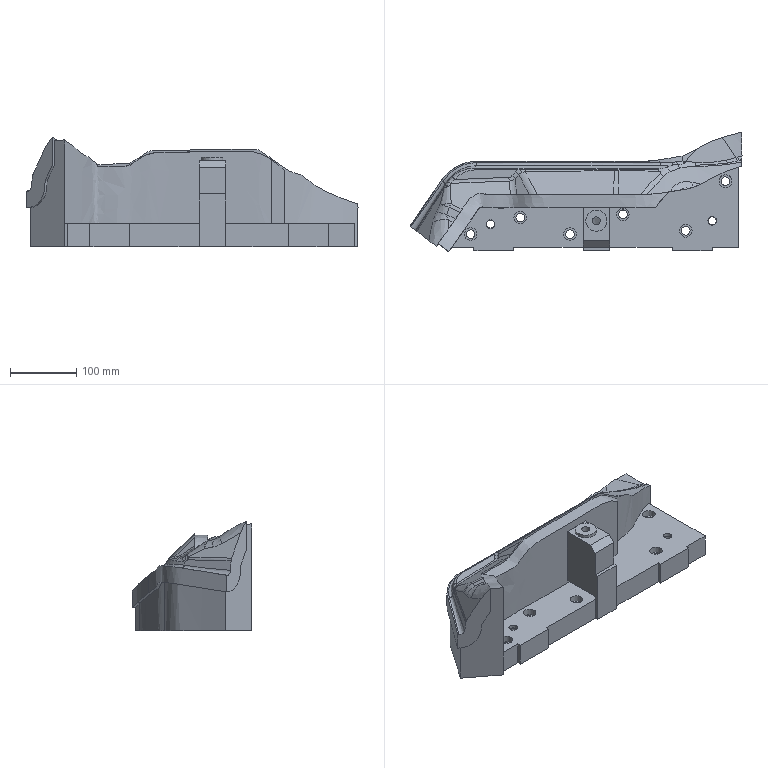Part | NX | features solid 2 | 1 solid | 141 faces | box 501.606 x 180.524 x 165.677 mm | volume 4989329 mm3 | spline 61 | plane 46 | cylinder 33 | cone 1 | commonest cylinder face diameters 13 x8 19 x6 40 x4 12 x3 20 x3 5.942 x1